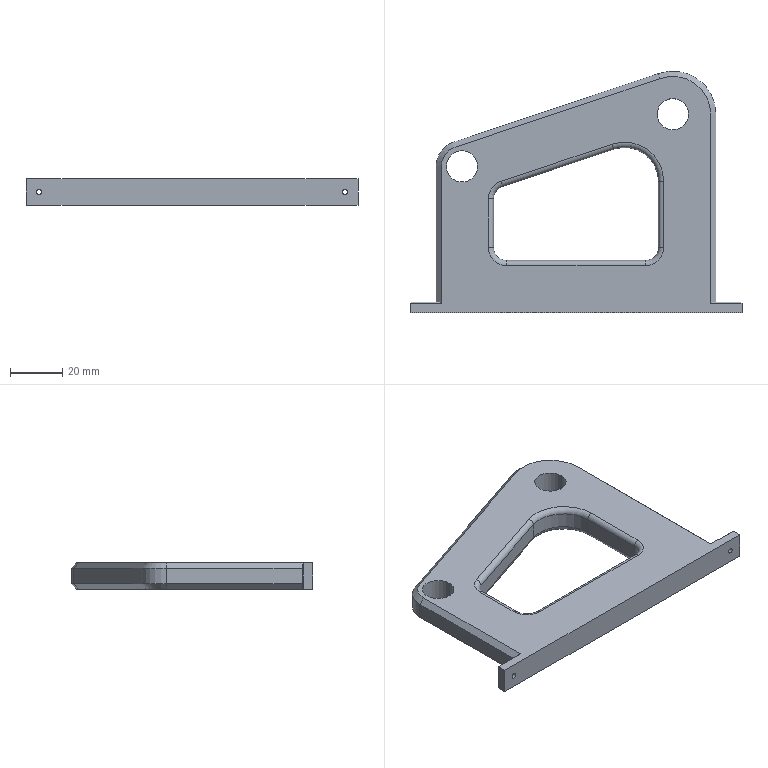Part | SolidWorks | features Fillet 3, Chamfer 2, ICE 2, Extrusion 1 | 1 solid | 60 faces | box 127.21 x 92.5 x 10 mm | volume 59705 mm3 | plane 26 | cylinder 22 | torus 8 | cone 4 | commonest cylinder face diameters 4 x8 2 x4 12 x4 10 x3 19.794 x1 26 x1